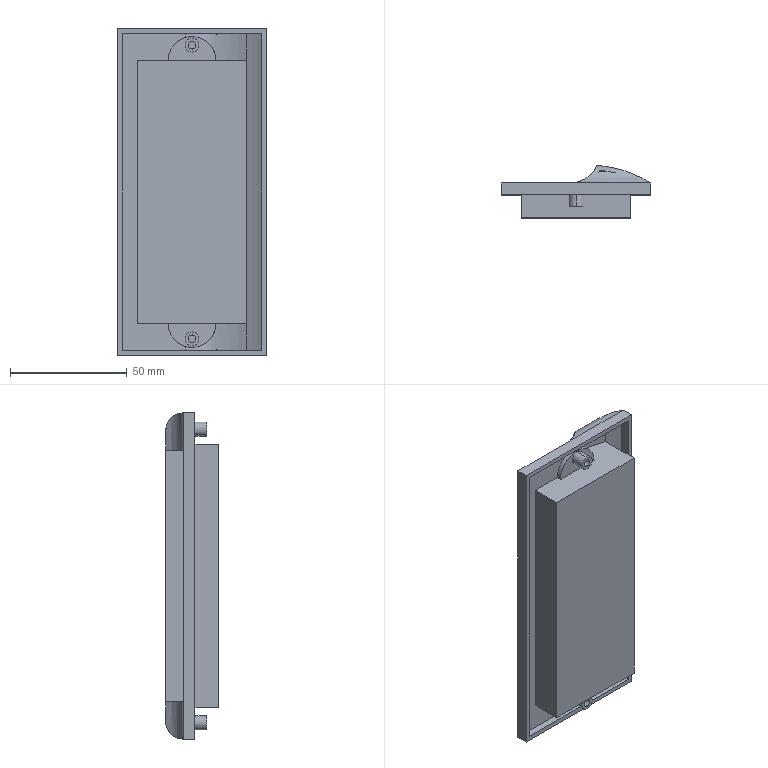Part | STEP file | XAM35_A140 | 1 solid | 49 faces | box 64 x 22.5 x 140 mm | volume 66990 mm3 | plane 29 | cylinder 20 | commonest cylinder face diameters 3.3 x4 6 x4 15 x2 20.36 x2 25.388 x2 29.388 x2